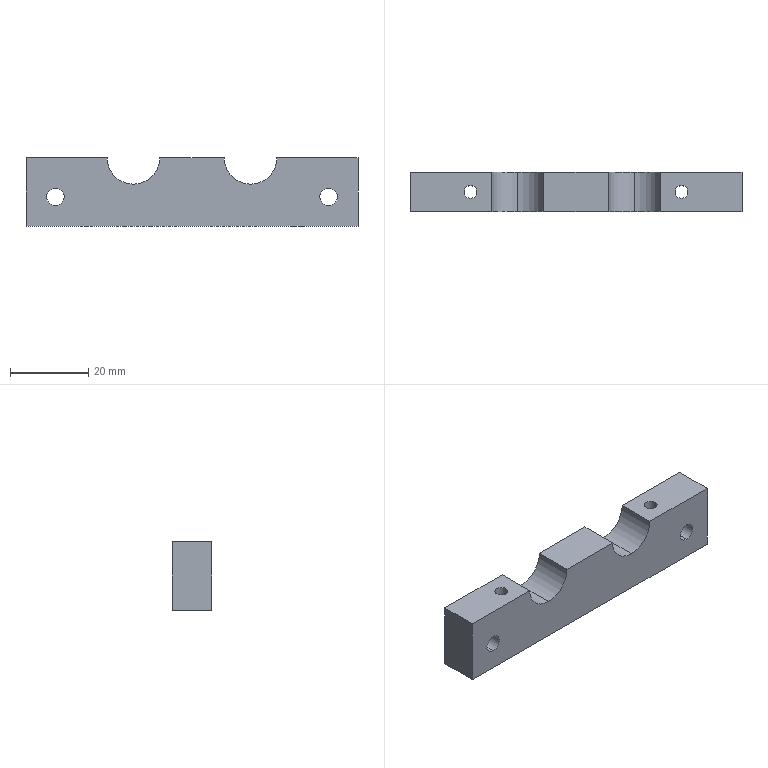Part | STEP file | Station two plug plate low | 1 solid | 26 faces | box 85 x 10 x 17.5 mm | volume 12524 mm3 | cylinder 16 | plane 10 | commonest cylinder face diameters 3.3 x4 4.5 x4 8 x4 13.5 x4